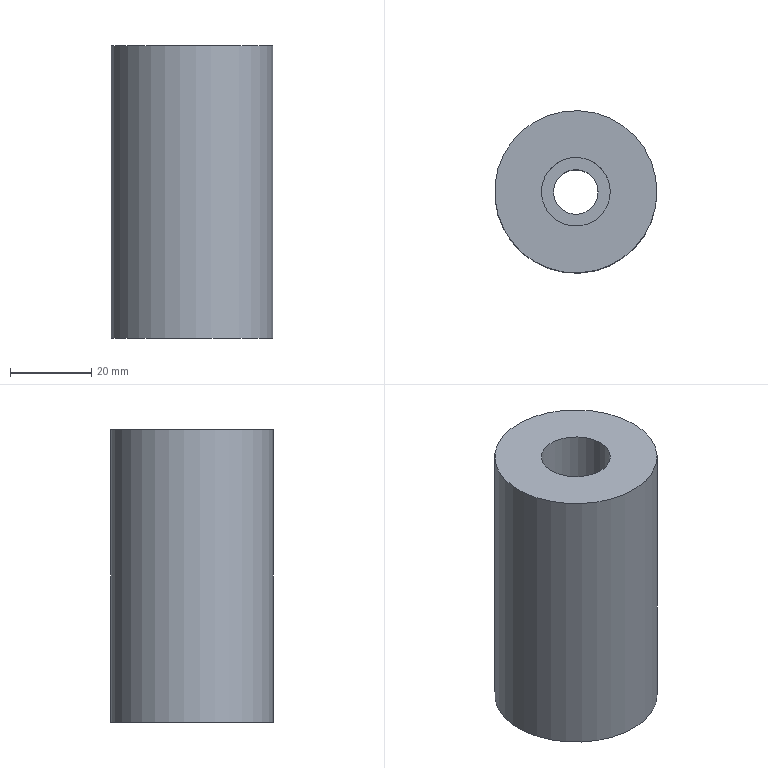Part | STEP file | 1 solid | 6 faces | box 40 x 40 x 72 mm | volume 79413 mm3 | plane 3 | cylinder 3 | commonest cylinder face diameters 11 x1 17 x1 40 x1
STEP:
#1=CARTESIAN_POINT('',(-325.,-157.5,25.));
#2=VERTEX_POINT('',#1);
#3=CARTESIAN_POINT('',(-345.,-157.5,25.));
#4=DIRECTION('',(0.,0.,-1.));
#5=DIRECTION('',(1.,0.,0.));
#6=AXIS2_PLACEMENT_3D('',#3,#4,#5);
#7=CIRCLE('',#6,20.);
#8=EDGE_CURVE('',#2,#2,#7,.T.);
#9=ORIENTED_EDGE('',*,*,#8,.F.);
#10=EDGE_LOOP('',(#9));
#11=FACE_BOUND('',#10,.T.);
#12=CARTESIAN_POINT('',(-336.5,-157.5,25.));
#13=VERTEX_POINT('',#12);
#14=CARTESIAN_POINT('',(-345.,-157.5,25.));
#15=DIRECTION('',(0.,0.,-1.));
#16=DIRECTION('',(1.,0.,0.));
#17=AXIS2_PLACEMENT_3D('',#14,#15,#16);
#18=CIRCLE('',#17,8.5);
#19=EDGE_CURVE('',#13,#13,#18,.T.);
#20=ORIENTED_EDGE('',*,*,#19,.T.);
#21=EDGE_LOOP('',(#20));
#22=FACE_BOUND('',#21,.T.);
#23=CARTESIAN_POINT('',(-345.,-157.5,25.));
#24=DIRECTION('',(0.,0.,1.));
#25=DIRECTION('',(1.,0.,0.));
#26=AXIS2_PLACEMENT_3D('',#23,#24,#25);
#27=PLANE('',#26);
#28=ADVANCED_FACE('',(#11,#22),#27,.T.);
#29=CARTESIAN_POINT('',(-325.,-157.5,-47.));
#30=VERTEX_POINT('',#29);
#31=CARTESIAN_POINT('',(-345.,-157.5,-47.));
#32=DIRECTION('',(0.,0.,1.));
#33=DIRECTION('',(1.,0.,0.));
#34=AXIS2_PLACEMENT_3D('',#31,#32,#33);
#35=CIRCLE('',#34,20.);
#36=EDGE_CURVE('',#30,#30,#35,.T.);
#37=ORIENTED_EDGE('',*,*,#36,.F.);
#38=EDGE_LOOP('',(#37));
#39=FACE_BOUND('',#38,.T.);
#40=CARTESIAN_POINT('',(-339.5,-157.5,-47.));
#41=VERTEX_POINT('',#40);
#42=CARTESIAN_POINT('',(-345.,-157.5,-47.));
#43=DIRECTION('',(0.,0.,1.));
#44=DIRECTION('',(1.,0.,0.));
#45=AXIS2_PLACEMENT_3D('',#42,#43,#44);
#46=CIRCLE('',#45,5.5);
#47=EDGE_CURVE('',#41,#41,#46,.T.);
#48=ORIENTED_EDGE('',*,*,#47,.T.);
#49=EDGE_LOOP('',(#48));
#50=FACE_BOUND('',#49,.T.);
#51=CARTESIAN_POINT('',(-345.,-157.5,-47.));
#52=DIRECTION('',(0.,0.,-1.));
#53=DIRECTION('',(-1.,0.,0.));
#54=AXIS2_PLACEMENT_3D('',#51,#52,#53);
#55=PLANE('',#54);
#56=ADVANCED_FACE('',(#39,#50),#55,.T.);
#57=ORIENTED_EDGE('',*,*,#8,.T.);
#58=EDGE_LOOP('',(#57));
#59=FACE_BOUND('',#58,.T.);
#60=ORIENTED_EDGE('',*,*,#36,.T.);
#61=EDGE_LOOP('',(#60));
#62=FACE_BOUND('',#61,.T.);
#63=CARTESIAN_POINT('',(-345.,-157.5,-47.));
#64=DIRECTION('',(0.,0.,1.));
#65=DIRECTION('',(1.,0.,0.));
#66=AXIS2_PLACEMENT_3D('',#63,#64,#65);
#67=CYLINDRICAL_SURFACE('',#66,20.);
#68=ADVANCED_FACE('',(#59,#62),#67,.T.);
#69=CARTESIAN_POINT('',(-350.5,-157.5,-7.));
#70=VERTEX_POINT('',#69);
#71=CARTESIAN_POINT('',(-345.,-157.5,-7.));
#72=DIRECTION('',(0.,0.,-1.));
#73=DIRECTION('',(-1.,0.,0.));
#74=AXIS2_PLACEMENT_3D('',#71,#72,#73);
#75=CIRCLE('',#74,5.5);
#76=EDGE_CURVE('',#70,#70,#75,.T.);
#77=ORIENTED_EDGE('',*,*,#76,.F.);
#78=EDGE_LOOP('',(#77));
#79=FACE_BOUND('',#78,.T.);
#80=ORIENTED_EDGE('',*,*,#47,.F.);
#81=EDGE_LOOP('',(#80));
#82=FACE_BOUND('',#81,.T.);
#83=CARTESIAN_POINT('',(-345.,-157.5,-47.));
#84=DIRECTION('',(0.,0.,1.));
#85=DIRECTION('',(1.,0.,0.));
#86=AXIS2_PLACEMENT_3D('',#83,#84,#85);
#87=CYLINDRICAL_SURFACE('',#86,5.5);
#88=ADVANCED_FACE('',(#79,#82),#87,.F.);
#89=ORIENTED_EDGE('',*,*,#76,.T.);
#90=EDGE_LOOP('',(#89));
#91=FACE_BOUND('',#90,.T.);
#92=CARTESIAN_POINT('',(-336.5,-157.5,-7.));
#93=VERTEX_POINT('',#92);
#94=CARTESIAN_POINT('',(-345.,-157.5,-7.));
#95=DIRECTION('',(0.,0.,-1.));
#96=DIRECTION('',(1.,0.,0.));
#97=AXIS2_PLACEMENT_3D('',#94,#95,#96);
#98=CIRCLE('',#97,8.5);
#99=EDGE_CURVE('',#93,#93,#98,.T.);
#100=ORIENTED_EDGE('',*,*,#99,.F.);
#101=EDGE_LOOP('',(#100));
#102=FACE_BOUND('',#101,.T.);
#103=CARTESIAN_POINT('',(-345.,-157.5,-7.));
#104=DIRECTION('',(0.,0.,-1.));
#105=DIRECTION('',(-1.,0.,0.));
#106=AXIS2_PLACEMENT_3D('',#103,#104,#105);
#107=PLANE('',#106);
#108=ADVANCED_FACE('',(#91,#102),#107,.F.);
#109=ORIENTED_EDGE('',*,*,#19,.F.);
#110=EDGE_LOOP('',(#109));
#111=FACE_BOUND('',#110,.T.);
#112=ORIENTED_EDGE('',*,*,#99,.T.);
#113=EDGE_LOOP('',(#112));
#114=FACE_BOUND('',#113,.T.);
#115=CARTESIAN_POINT('',(-345.,-157.5,-7.));
#116=DIRECTION('',(0.,0.,1.));
#117=DIRECTION('',(1.,0.,0.));
#118=AXIS2_PLACEMENT_3D('',#115,#116,#117);
#119=CYLINDRICAL_SURFACE('',#118,8.5);
#120=ADVANCED_FACE('',(#111,#114),#119,.F.);
#121=CLOSED_SHELL('',(#28,#56,#68,#88,#108,#120));
#122=MANIFOLD_SOLID_BREP('',#121);
#123=(LENGTH_UNIT()NAMED_UNIT(*)SI_UNIT(.MILLI.,.METRE.));
#124=UNCERTAINTY_MEASURE_WITH_UNIT(LENGTH_MEASURE(0.00002),#123,'','');
#125=(NAMED_UNIT(*)PLANE_ANGLE_UNIT()SI_UNIT($,.RADIAN.));
#126=PLANE_ANGLE_MEASURE_WITH_UNIT(PLANE_ANGLE_MEASURE(0.01745),#125);
#127=DIMENSIONAL_EXPONENTS(0.,0.,0.,0.,0.,0.,0.);
#128=(CONVERSION_BASED_UNIT('DEGREE',#126)NAMED_UNIT(#127)PLANE_ANGLE_UNIT());
#129=(NAMED_UNIT(*)SI_UNIT($,.STERADIAN.)SOLID_ANGLE_UNIT());
#130=(GEOMETRIC_REPRESENTATION_CONTEXT(3)GLOBAL_UNCERTAINTY_ASSIGNED_CONTEXT((#124))GLOBAL_UNIT_ASSIGNED_CONTEXT((#123,#128,#129))REPRESENTATION_CONTEXT('',''));
#131=ADVANCED_BREP_SHAPE_REPRESENTATION('',(#122),#130);